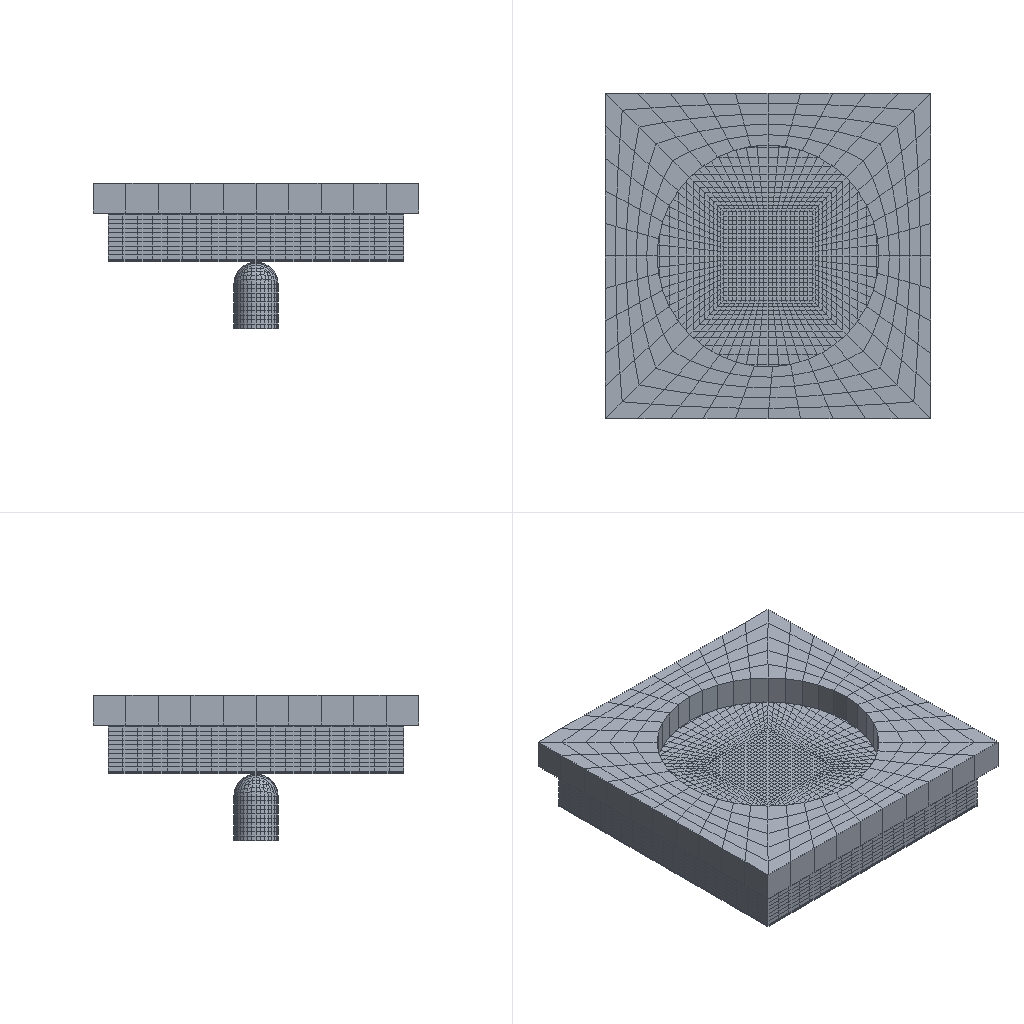Simulation study | abaqus
Set-up summary:
category,name,step,type,value,unit,region
solver,abaqus
solver,version,,,Abaqus/Explicit 2020
units,not stated in the deck,,not stated
analysis,deck,,transient,transient
load_step,Step-1,Step-1,transient
load_step,requested,,,1
mesh,nodes,,,44372
mesh,elements,,,36568
element_type,SC8R,,solid_shell,18240
element_type,C3D8R,,solid,16808
element_type,COH3D8,,cohesive,1520
load,load commands in deck,,count,1
bc,support commands in deck,,count,12
material,CFRP,,in results
material,GANGTI,,in results
material,JIAO,,in results
material,PMI,,in results
check,setup vs results,,match,"per instance, exact: element labels, types and connectivity; labels of the nodes the elements use; coordinates not compared"
Abaqus input file, long lists of numbers shortened:
*Heading
** Job name: Job-1 Model name: Model-1
** Generated by: Abaqus/CAE 2020
*Preprint, echo=NO, model=NO, history=NO, contact=NO
**
** PARTS
**
*Part, name=boligang
*Node
      1,         -25.,          55.,           0.
      2,          10.,          90.,           0.
** (17169 more lines like these left out)
*Element, type=C3D8R
1521,    1,    9,  213,   72, 1562, 1570, 1774, 1633
1522,    9,   10,  214,  213, 1570, 1571, 1775, 1774
** (15198 more lines like these left out)
*Elset, elset=eleset1, generate
 1521,  3040,     1
*Elset, elset=eleset2, generate
 3041,  4560,     1
*Elset, elset=eleset3, generate
 4561,  6080,     1
*Elset, elset=eleset4, generate
 6081,  7600,     1
*Elset, elset=eleset5, generate
 7601,  9120,     1
*Elset, elset=eleset6, generate
  9121,  10640,      1
*Elset, elset=eleset7, generate
 10641,  12160,      1
*Elset, elset=eleset8, generate
 12161,  13680,      1
*Elset, elset=eleset9, generate
 13681,  15200,      1
*Elset, elset=eleset10, generate
 15201,  16720,      1
*Elset, elset=all_plate_elems, generate
  1521,  16720,      1
*Elset, elset=paomo, generate
  1521,  16720,      1
*Elset, elset=_plate_interior_surf_S1, internal, generate
  1521,  16720,      1
*Elset, elset=_plate_interior_surf_S2, internal, generate
  1521,  16720,      1
*Elset, elset=_plate_interior_surf_S3, internal, generate
  1521,  16720,      1
*Elset, elset=_plate_interior_surf_S4, internal, generate
  1521,  16720,      1
*Elset, elset=_plate_interior_surf_S5, internal, generate
  1521,  16720,      1
*Elset, elset=_plate_interior_surf_S6, internal, generate
  1521,  16720,      1
*Surface, type=ELEMENT, name=plate_interior_surf
_plate_interior_surf_S1, S1
_plate_interior_surf_S2, S2
_plate_interior_surf_S4, S4
_plate_interior_surf_S6, S6
_plate_interior_surf_S3, S3
_plate_interior_surf_S5, S5
*Orientation, name=Ori-1
          1.,           0.,           0.,           0.,           1.,           0.
3, 0.
** Section: pmi0
*Solid Section, elset=eleset1, orientation=Ori-1, controls=EC-3, material=pmi
,
*Orientation, name=Ori-2
          1.,           0.,           0.,           0.,           1.,           0.
3, 0.
** Section: pmi0
*Solid Section, elset=eleset2, orientation=Ori-2, controls=EC-3, material=pmi
,
*Orientation, name=Ori-3
          1.,           0.,           0.,           0.,           1.,           0.
3, 0.
** Section: pmi0
*Solid Section, elset=eleset3, orientation=Ori-3, controls=EC-3, material=pmi
,
*Orientation, name=Ori-4
          1.,           0.,           0.,           0.,           1.,           0.
3, 0.
** Section: pmi0
*Solid Section, elset=eleset4, orientation=Ori-4, controls=EC-3, material=pmi
,
*Orientation, name=Ori-5
          1.,           0.,           0.,           0.,           1.,           0.
3, 0.
** Section: pmi0
*Solid Section, elset=eleset5, orientation=Ori-5, controls=EC-3, material=pmi
,
*Orientation, name=Ori-6
          1.,           0.,           0.,           0.,           1.,           0.
3, 0.
** Section: pmi0
*Solid Section, elset=eleset6, orientation=Ori-6, controls=EC-3, material=pmi
,
*Orientation, name=Ori-7
          1.,           0.,           0.,           0.,           1.,           0.
3, 0.
** Section: pmi0
*Solid Section, elset=eleset7, orientation=Ori-7, controls=EC-3, material=pmi
,
*Orientation, name=Ori-8
          1.,           0.,           0.,           0.,           1.,           0.
3, 0.
** Section: pmi0
*Solid Section, elset=eleset8, orientation=Ori-8, controls=EC-3, material=pmi
,
*Orientation, name=Ori-9
          1.,           0.,           0.,           0.,           1.,           0.
3, 0.
** Section: pmi0
*Solid Section, elset=eleset9, orientation=Ori-9, controls=EC-3, material=pmi
,
*Orientation, name=Ori-10
          1.,           0.,           0.,           0.,           1.,           0.
3, 0.
** Region: (pmi0:eleset10), (Controls:EC-3), (Material Orientation:eleset10)
*Elset, elset=_I10, internal
 15201, 15202, 15203, 15204, 15205, 15206, 15207, 15208, 15209, 15210, 15211, 15212, 15213, 15215, 15216, 15217
 15218, 15219, 15220, 15221, 15222, 15223, 15224, 15225, 15226, 15227, 15228, 15229, 15230, 15231, 15232, 15233
** (93 more lines like these left out)
** Section: pmi0
*Solid Section, elset=_I10, orientation=Ori-10, controls=EC-3, material=pmi
,
** Region: (pmi0:eleset10), (Controls:Default), (Material Orientation:eleset10)
*Elset, elset=_I11, internal
 15214,
** Section: pmi0
*Solid Section, elset=_I11, orientation=Ori-10, material=pmi
,
*End Part
**
*Part, name=chongtou
*Node
      1,           0.,           0.,           0.
      2,           0.,           0.,         -7.5
** (1742 more lines like these left out)
*Element, type=C3D8R
  1, 209, 210, 950, 932,  15,  14, 178, 177
  2, 210, 211, 951, 950,  14,  13, 179, 178
** (1406 more lines like these left out)
*Node
   1745,           0.,         -7.5,           0.
*Nset, nset=chongtou-RefPt_, internal
1745,
*Nset, nset=_PickedSet3, internal, generate
    1,  1744,     1
*Elset, elset=_PickedSet3, internal, generate
    1,  1408,     1
** Section: gangti
*Solid Section, elset=_PickedSet3, material=gangti
,
*End Part
**
*Part, name=jiaju
*Node
      1,         -85.,         92.5,          10.
      2,          25.,         92.5,          10.
** (478 more lines like these left out)
*Element, type=C3D8R
 1,  62, 193, 229,  55,   1,  19,  36,   4
 2, 193, 194, 230, 229,  19,  20,  35,  36
** (198 more lines like these left out)
*Nset, nset=_PickedSet2, internal, generate
   1,  480,    1
*Elset, elset=_PickedSet2, internal, generate
   1,  200,    1
** Section: gangti
*Solid Section, elset=_PickedSet2, material=gangti
,
*End Part
**
*Part, name=jiao
*Node
      1,         -25.,          55.,           0.
      2,          10.,          90.,           0.
** (3120 more lines like these left out)
*Element, type=COH3D8
1521,    1,    9,  213,   72, 1562, 1570, 1774, 1633
1522,    9,   10,  214,  213, 1570, 1571, 1775, 1774
** (1518 more lines like these left out)
*Elset, elset=jiao, generate
 1521,  3040,     1
*Elset, elset=_PickedSet10, internal, generate
 1521,  3040,     1
*Elset, elset=jiaoshang, generate
 1521,  3040,     1
*Elset, elset=jiaoxia, generate
 1521,  3040,     1
** Section: jiao
*Cohesive Section, elset=_PickedSet10, controls=EC-2, material=jiao, response=TRACTION SEPARATION
,
*End Part
**
*Part, name=mianban
*Node
      1,         -25.,          55.,           0.
      2,          10.,          90.,           0.
** (10925 more lines like these left out)
*Element, type=SC8R
1521,    1,    9,  213,   72, 1562, 1570, 1774, 1633
1522,    9,   10,  214,  213, 1570, 1571, 1775, 1774
** (9118 more lines like these left out)
*Elset, elset=eleset1, generate
 1521,  3040,     1
*Elset, elset=eleset2, generate
 3041,  4560,     1
*Elset, elset=eleset3, generate
 4561,  6080,     1
*Elset, elset=eleset4, generate
 6081,  7600,     1
*Elset, elset=eleset5, generate
 7601,  9120,     1
*Elset, elset=eleset6, generate
  9121,  10640,      1
*Nset, nset=yueshu
    2,    3,    6,    8,   22,   23,   24,   25,   26,   27,   28,   29,   30,   31,   32,   33
   34,   35,   36,   37,   38,   39,   40,   86,   87,   88,   89,   90,   91,   92,   93,   94
** (33 more lines like these left out)
*Elset, elset=ban, generate
  1521,  10640,      1
*Elset, elset=shang, generate
  1521,  10640,      1
*Elset, elset=_inner_S1, internal
  2641,  2642,  2643,  2644,  2645,  2646,  2647,  2648,  2649,  2650,  2651,  2652,  2653,  2654,  2655,  2656
  2657,  2658,  2659,  2660,  2661,  2662,  2663,  2664,  2665,  2666,  2667,  2668,  2669,  2670,  2671,  2672
** (148 more lines like these left out)
*Elset, elset=_inner_S2, internal
  2641,  2642,  2643,  2644,  2645,  2646,  2647,  2648,  2649,  2650,  2651,  2652,  2653,  2654,  2655,  2656
  2657,  2658,  2659,  2660,  2661,  2662,  2663,  2664,  2665,  2666,  2667,  2668,  2669,  2670,  2671,  2672
** (148 more lines like these left out)
*Elset, elset=_inner_S3, internal
  2661,  2662,  2663,  2664,  2665,  2666,  2667,  2668,  2669,  2670,  2671,  2672,  2673,  2674,  2675,  2676
  2677,  2678,  2679,  2680,  2681,  2682,  2683,  2684,  2685,  2686,  2687,  2688,  2689,  2690,  2691,  2692
** (141 more lines like these left out)
*Elset, elset=_inner_S4, internal
  2641,  2642,  2643,  2644,  2645,  2646,  2647,  2648,  2649,  2650,  2651,  2652,  2653,  2654,  2655,  2656
  2657,  2658,  2659,  2661,  2662,  2663,  2664,  2665,  2666,  2667,  2668,  2669,  2670,  2671,  2672,  2673
** (141 more lines like these left out)
*Elset, elset=_inner_S5, internal
  2641,  2642,  2643,  2644,  2645,  2646,  2647,  2648,  2649,  2650,  2651,  2652,  2653,  2654,  2655,  2656
  2657,  2658,  2659,  2660,  2661,  2662,  2663,  2664,  2665,  2666,  2667,  2668,  2669,  2670,  2671,  2672
** (141 more lines like these left out)
*Elset, elset=_inner_S6, internal
  2642,  2643,  2644,  2645,  2646,  2647,  2648,  2649,  2650,  2651,  2652,  2653,  2654,  2655,  2656,  2657
  2658,  2659,  2660,  2662,  2663,  2664,  2665,  2666,  2667,  2668,  2669,  2670,  2671,  2672,  2673,  2674
** (141 more lines like these left out)
*Surface, type=ELEMENT, name=inner
_inner_S1, S1
_inner_S2, S2
_inner_S4, S4
_inner_S6, S6
_inner_S3, S3
_inner_S5, S5
*Orientation, name=Ori-1
          1.,           0.,           0.,           0.,           1.,           0.
3, 0.
** Region: (CompositeLayup-1-1: Generated From Layup), (Controls:EC-1)
*Elset, elset=CompositeLayup-1-1, generate
 1521,  3040,     1
** Section: CompositeLayup-1-1
*Shell Section, elset=CompositeLayup-1-1, composite, orientation=Ori-1, controls=EC-1, stack direction=3, layup=CompositeLayup-1
0.125, 3, cfrp, 0., Ply-1
*Orientation, name=Ori-4
          1.,           0.,           0.,           0.,           1.,           0.
3, 0.
** Region: (CompositeLayup-1-4: Generated From Layup), (Controls:EC-1)
*Elset, elset=CompositeLayup-1-4, generate
 3041,  4560,     1
** Section: CompositeLayup-1-4
*Shell Section, elset=CompositeLayup-1-4, composite, orientation=Ori-4, controls=EC-1, stack direction=3, layup=CompositeLayup-1
0.125, 3, cfrp, 90., Ply-2
*Orientation, name=Ori-2
          1.,           0.,           0.,           0.,           1.,           0.
3, 0.
** Region: (CompositeLayup-1-2: Generated From Layup), (Controls:EC-1)
*Elset, elset=CompositeLayup-1-2, generate
 4561,  6080,     1
** Section: CompositeLayup-1-2
*Shell Section, elset=CompositeLayup-1-2, composite, orientation=Ori-2, controls=EC-1, stack direction=3, layup=CompositeLayup-1
0.125, 3, cfrp, 0., Ply-3
*Orientation, name=Ori-5
          1.,           0.,           0.,           0.,           1.,           0.
3, 0.
** Region: (CompositeLayup-1-5: Generated From Layup), (Controls:EC-1)
*Elset, elset=CompositeLayup-1-5, generate
 6081,  7600,     1
** Section: CompositeLayup-1-5
*Shell Section, elset=CompositeLayup-1-5, composite, orientation=Ori-5, controls=EC-1, stack direction=3, layup=CompositeLayup-1
0.125, 3, cfrp, 90., Ply-4
*Orientation, name=Ori-3
          1.,           0.,           0.,           0.,           1.,           0.
3, 0.
** Region: (CompositeLayup-1-3: Generated From Layup), (Controls:EC-1)
*Elset, elset=CompositeLayup-1-3, generate
 7601,  9120,     1
** Section: CompositeLayup-1-3
*Shell Section, elset=CompositeLayup-1-3, composite, orientation=Ori-3, controls=EC-1, stack direction=3, layup=CompositeLayup-1
0.125, 3, cfrp, 0., Ply-5
*Orientation, name=Ori-6
          1.,           0.,           0.,           0.,           1.,           0.
3, 0.
** Region: (CompositeLayup-1-6: Generated From Layup), (Controls:EC-1)
*Elset, elset=CompositeLayup-1-6, generate
  9121,  10640,      1
** Section: CompositeLayup-1-6
*Shell Section, elset=CompositeLayup-1-6, composite, orientation=Ori-6, controls=EC-1, stack direction=3, layup=CompositeLayup-1
0.125, 3, cfrp, 90., Ply-6
*End Part
**
*Part, name=mianban2
*Node
      1,         -25.,          55.,           0.
      2,          10.,          90.,           0.
** (10925 more lines like these left out)
*Element, type=SC8R
1521,    1,    9,  213,   72, 1562, 1570, 1774, 1633
1522,    9,   10,  214,  213, 1570, 1571, 1775, 1774
** (9118 more lines like these left out)
*Elset, elset=eleset1, generate
 1521,  3040,     1
*Elset, elset=eleset2, generate
 3041,  4560,     1
*Elset, elset=eleset3, generate
 4561,  6080,     1
*Elset, elset=eleset4, generate
 6081,  7600,     1
*Elset, elset=eleset5, generate
 7601,  9120,     1
*Elset, elset=eleset6, generate
  9121,  10640,      1
*Elset, elset=ban, generate
  1521,  10640,      1
*Nset, nset=yueshu
    2,    3,    6,    8,   22,   23,   24,   25,   26,   27,   28,   29,   30,   31,   32,   33
   34,   35,   36,   37,   38,   39,   40,   86,   87,   88,   89,   90,   91,   92,   93,   94
** (33 more lines like these left out)
*Elset, elset=xia, generate
  1521,  10640,      1
*Elset, elset=_inner_S1, internal
  2641,  2642,  2643,  2644,  2645,  2646,  2647,  2648,  2649,  2650,  2651,  2652,  2653,  2654,  2655,  2656
  2657,  2658,  2659,  2660,  2661,  2662,  2663,  2664,  2665,  2666,  2667,  2668,  2669,  2670,  2671,  2672
** (148 more lines like these left out)
*Elset, elset=_inner_S2, internal
  2641,  2642,  2643,  2644,  2645,  2646,  2647,  2648,  2649,  2650,  2651,  2652,  2653,  2654,  2655,  2656
  2657,  2658,  2659,  2660,  2661,  2662,  2663,  2664,  2665,  2666,  2667,  2668,  2669,  2670,  2671,  2672
** (148 more lines like these left out)
*Elset, elset=_inner_S3, internal
  2661,  2662,  2663,  2664,  2665,  2666,  2667,  2668,  2669,  2670,  2671,  2672,  2673,  2674,  2675,  2676
  2677,  2678,  2679,  2680,  2681,  2682,  2683,  2684,  2685,  2686,  2687,  2688,  2689,  2690,  2691,  2692
** (141 more lines like these left out)
*Elset, elset=_inner_S4, internal
  2641,  2642,  2643,  2644,  2645,  2646,  2647,  2648,  2649,  2650,  2651,  2652,  2653,  2654,  2655,  2656
  2657,  2658,  2659,  2661,  2662,  2663,  2664,  2665,  2666,  2667,  2668,  2669,  2670,  2671,  2672,  2673
** (141 more lines like these left out)
*Elset, elset=_inner_S5, internal
  2641,  2642,  2643,  2644,  2645,  2646,  2647,  2648,  2649,  2650,  2651,  2652,  2653,  2654,  2655,  2656
  2657,  2658,  2659,  2660,  2661,  2662,  2663,  2664,  2665,  2666,  2667,  2668,  2669,  2670,  2671,  2672
** (141 more lines like these left out)
*Elset, elset=_inner_S6, internal
  2642,  2643,  2644,  2645,  2646,  2647,  2648,  2649,  2650,  2651,  2652,  2653,  2654,  2655,  2656,  2657
  2658,  2659,  2660,  2662,  2663,  2664,  2665,  2666,  2667,  2668,  2669,  2670,  2671,  2672,  2673,  2674
** (141 more lines like these left out)
*Surface, type=ELEMENT, name=inner
_inner_S1, S1
_inner_S2, S2
_inner_S4, S4
_inner_S6, S6
_inner_S3, S3
_inner_S5, S5
*Orientation, name=Ori-1
          1.,           0.,           0.,           0.,           1.,           0.
3, 0.
** Region: (CompositeLayup-1-1: Generated From Layup), (Controls:EC-1)
*Elset, elset=CompositeLayup-1-1, generate
 1521,  3040,     1
** Section: CompositeLayup-1-1
*Shell Section, elset=CompositeLayup-1-1, composite, orientation=Ori-1, controls=EC-1, stack direction=3, layup=CompositeLayup-1
0.125, 3, cfrp, 0., Ply-1
*Orientation, name=Ori-4
          1.,           0.,           0.,           0.,           1.,           0.
3, 0.
** Region: (CompositeLayup-1-4: Generated From Layup), (Controls:EC-1)
*Elset, elset=CompositeLayup-1-4, generate
 3041,  4560,     1
** Section: CompositeLayup-1-4
*Shell Section, elset=CompositeLayup-1-4, composite, orientation=Ori-4, controls=EC-1, stack direction=3, layup=CompositeLayup-1
0.125, 3, cfrp, 90., Ply-2
*Orientation, name=Ori-2
          1.,           0.,           0.,           0.,           1.,           0.
3, 0.
** Region: (CompositeLayup-1-2: Generated From Layup), (Controls:EC-1)
*Elset, elset=CompositeLayup-1-2, generate
 4561,  6080,     1
** Section: CompositeLayup-1-2
*Shell Section, elset=CompositeLayup-1-2, composite, orientation=Ori-2, controls=EC-1, stack direction=3, layup=CompositeLayup-1
0.125, 3, cfrp, 0., Ply-3
*Orientation, name=Ori-5
          1.,           0.,           0.,           0.,           1.,           0.
3, 0.
** Region: (CompositeLayup-1-5: Generated From Layup), (Controls:EC-1)
*Elset, elset=CompositeLayup-1-5, generate
 6081,  7600,     1
** Section: CompositeLayup-1-5
*Shell Section, elset=CompositeLayup-1-5, composite, orientation=Ori-5, controls=EC-1, stack direction=3, layup=CompositeLayup-1
0.125, 3, cfrp, 90., Ply-4
*Orientation, name=Ori-3
          1.,           0.,           0.,           0.,           1.,           0.
3, 0.
** Region: (CompositeLayup-1-3: Generated From Layup), (Controls:EC-1)
*Elset, elset=CompositeLayup-1-3, generate
 7601,  9120,     1
** Section: CompositeLayup-1-3
*Shell Section, elset=CompositeLayup-1-3, composite, orientation=Ori-3, controls=EC-1, stack direction=3, layup=CompositeLayup-1
0.125, 3, cfrp, 0., Ply-5
*Orientation, name=Ori-6
          1.,           0.,           0.,           0.,           1.,           0.
3, 0.
** Region: (CompositeLayup-1-6: Generated From Layup), (Controls:EC-1)
*Elset, elset=CompositeLayup-1-6, generate
  9121,  10640,      1
** Section: CompositeLayup-1-6
*Shell Section, elset=CompositeLayup-1-6, composite, orientation=Ori-6, controls=EC-1, stack direction=3, layup=CompositeLayup-1
0.125, 3, cfrp, 90., Ply-6
*End Part
**
**
** ASSEMBLY
**
*Assembly, name=Assembly
**
*Instance, name=chongtou-1, part=chongtou
        -35.,         42.5,       -24.05
        -35.,         42.5,       -24.05, -36.,         42.5,       -24.05, 90.
*End Instance
**
*Instance, name=jiaju-1, part=jiaju
         -5.,           5.,           0.
*End Instance
**
*Instance, name=mianban-1, part=mianban
          5.,          2.5,        -16.5
*End Instance
**
*Instance, name=mianban2-1, part=mianban2
          5.,          2.5,        -0.75
*End Instance
**
*Instance, name=jiao-1, part=jiao
          5.,          2.5,       -15.75
*End Instance
**
*Instance, name=boligang-1, part=boligang
          5.,          2.5,       -15.65
*End Instance
**
*Node
      1,         -35.,         42.5,          10.
*Elset, elset=ban, instance=mianban2-1, generate
  1521,  10640,      1
*Nset, nset=tou, instance=chongtou-1
 1745,
*Nset, nset=_PickedSet13, internal, instance=chongtou-1
 1745,
*Nset, nset=_PickedSet17, internal
 1,
*Nset, nset=_PickedSet18, internal, instance=jiaju-1, generate
   1,  480,    1
*Elset, elset=_PickedSet18, internal, instance=jiaju-1, generate
   1,  200,    1
*Nset, nset=_PickedSet19, internal
 1,
*Nset, nset=_PickedSet20, internal, instance=chongtou-1
 1745,
*Nset, nset=_PickedSet44, internal, instance=chongtou-1, generate
    1,  1744,     1
*Elset, elset=_PickedSet44, internal, instance=chongtou-1, generate
    1,  1408,     1
*Nset, nset=_PickedSet83, internal, instance=mianban2-1
    2,    3,    6,    8,   22,   23,   24,   25,   26,   27,   28,   29,   30,   31,   32,   33
   34,   35,   36,   37,   38,   39,   40,   86,   87,   88,   89,   90,   91,   92,   93,   94
** (33 more lines like these left out)
*Nset, nset=_PickedSet83, internal, instance=boligang-1
     2,     3,     6,     8,    22,    23,    24,    25,    26,    27,    28,    29,    30,    31,    32,    33
    34,    35,    36,    37,    38,    39,    40,    86,    87,    88,    89,    90,    91,    92,    93,    94
** (53 more lines like these left out)
*Elset, elset=_inner_S1, internal, instance=mianban2-1
  1521,  1522,  1523,  1524,  1535,  1536,  1537,  1538,  1549,  1550,  1551,  1552,  1563,  1564,  1565,  1566
  1577,  1578,  1579,  1580,  1591,  1592,  1593,  1594,  1605,  1606,  1607,  1608,  1619,  1620,  1621,  1622
** (268 more lines like these left out)
*Elset, elset=_inner_S1, internal, instance=boligang-1
  1521,  1522,  1523,  1535,  1536,  1537,  1549,  1550,  1551,  1563,  1564,  1565,  1577,  1578,  1579,  1591
  1592,  1593,  1605,  1606,  1607,  1619,  1620,  1621,  1633,  1634,  1635,  1647,  1648,  1649,  1661,  1662
** (426 more lines like these left out)
*Elset, elset=_inner_S2, internal, instance=mianban2-1
  1521,  1522,  1523,  1524,  1535,  1536,  1537,  1538,  1549,  1550,  1551,  1552,  1563,  1564,  1565,  1566
  1577,  1578,  1579,  1580,  1591,  1592,  1593,  1594,  1605,  1606,  1607,  1608,  1619,  1620,  1621,  1622
** (268 more lines like these left out)
*Elset, elset=_inner_S2, internal, instance=boligang-1
  1521,  1522,  1523,  1535,  1536,  1537,  1549,  1550,  1551,  1563,  1564,  1565,  1577,  1578,  1579,  1591
  1592,  1593,  1605,  1606,  1607,  1619,  1620,  1621,  1633,  1634,  1635,  1647,  1648,  1649,  1661,  1662
** (431 more lines like these left out)
*Elset, elset=_inner_S3, internal, instance=mianban2-1
  1521,  1522,  1523,  1535,  1536,  1537,  1538,  1549,  1550,  1551,  1552,  1563,  1564,  1565,  1566,  1577
  1578,  1579,  1580,  1591,  1592,  1593,  1594,  1605,  1606,  1607,  1608,  1619,  1620,  1621,  1622,  1633
** (267 more lines like these left out)
*Elset, elset=_inner_S3, internal, instance=boligang-1
  1521,  1522,  1523,  1535,  1536,  1537,  1549,  1550,  1551,  1563,  1564,  1565,  1577,  1578,  1579,  1591
  1592,  1593,  1605,  1606,  1607,  1619,  1620,  1621,  1633,  1634,  1635,  1647,  1648,  1649,  1661,  1662
** (430 more lines like these left out)
*Elset, elset=_inner_S4, internal, instance=mianban2-1
  1521,  1522,  1523,  1535,  1536,  1537,  1549,  1550,  1551,  1563,  1564,  1565,  1577,  1578,  1579,  1591
  1592,  1593,  1605,  1606,  1607,  1619,  1620,  1621,  1633,  1634,  1635,  1647,  1648,  1649,  1661,  1662
** (253 more lines like these left out)
*Elset, elset=_inner_S4, internal, instance=boligang-1
  1521,  1522,  1535,  1536,  1549,  1550,  1563,  1564,  1577,  1578,  1591,  1592,  1605,  1606,  1619,  1620
  1633,  1634,  1647,  1648,  1661,  1662,  1675,  1676,  1689,  1690,  1703,  1704,  1717,  1718,  1731,  1732
** (406 more lines like these left out)
*Elset, elset=_inner_S5, internal, instance=mianban2-1
  1521,  1522,  1523,  1524,  1535,  1536,  1537,  1538,  1549,  1550,  1551,  1552,  1563,  1564,  1565,  1566
  1577,  1578,  1579,  1580,  1591,  1592,  1593,  1594,  1605,  1606,  1607,  1608,  1619,  1620,  1621,  1622
** (268 more lines like these left out)
*Elset, elset=_inner_S5, internal, instance=boligang-1
  1521,  1522,  1523,  1535,  1536,  1537,  1549,  1550,  1551,  1563,  1564,  1565,  1577,  1578,  1579,  1591
  1592,  1593,  1605,  1606,  1607,  1619,  1620,  1621,  1633,  1634,  1635,  1647,  1648,  1649,  1661,  1662
** (430 more lines like these left out)
*Elset, elset=_inner_S6, internal, instance=mianban2-1
  1521,  1522,  1523,  1524,  1535,  1536,  1537,  1538,  1549,  1550,  1551,  1552,  1563,  1564,  1565,  1566
  1577,  1578,  1579,  1580,  1591,  1592,  1593,  1594,  1605,  1606,  1607,  1608,  1619,  1620,  1621,  1622
** (253 more lines like these left out)
*Elset, elset=_inner_S6, internal, instance=boligang-1
  1521,  1522,  1523,  1535,  1536,  1537,  1549,  1550,  1551,  1563,  1564,  1565,  1577,  1578,  1579,  1591
  1592,  1593,  1605,  1606,  1607,  1619,  1620,  1621,  1633,  1634,  1635,  1647,  1648,  1649,  1661,  1662
** (406 more lines like these left out)
*Surface, type=ELEMENT, name=inner
_inner_S1, S1
_inner_S2, S2
_inner_S4, S4
_inner_S6, S6
_inner_S3, S3
_inner_S5, S5
*Elset, elset=_mian_S3, internal, instance=chongtou-1
   65,   66,   67,   68,   69,   70,   71,   72,   73,   74,   75,   76,   77,   78,   79,   80
   97,   98,   99,  100,  101,  102,  103,  104,  105,  106,  107,  108,  109,  110,  111,  112
** (2 more lines like these left out)
*Elset, elset=_mian_S4, internal, instance=chongtou-1
   81,   82,   83,   84,   85,   86,   87,   88,   89,   90,   91,   92,   93,   94,   95,   96
  465,  466,  467,  468,  469,  470,  471,  472,  473,  474,  475,  476,  477,  478,  479,  480
** (3 more lines like these left out)
*Elset, elset=_mian_S2, internal, instance=chongtou-1, generate
 353,  400,    1
*Surface, type=ELEMENT, name=mian
_mian_S3, S3
_mian_S4, S4
_mian_S2, S2
*Elset, elset=_s_Surf-9_S2, internal, instance=jiao-1, generate
 1521,  3040,     1
*Surface, type=ELEMENT, name=s_Surf-9
_s_Surf-9_S2, S2
*Elset, elset=__PickedSurf71_S1, internal, instance=boligang-1, generate
 1521,  3040,     1
*Surface, type=ELEMENT, name=_PickedSurf71, internal
__PickedSurf71_S1, S1
*Elset, elset=__PickedSurf75_S2, internal, instance=boligang-1, generate
 15201,  16720,      1
*Surface, type=ELEMENT, name=_PickedSurf75, internal
__PickedSurf75_S2, S2
*Elset, elset=__PickedSurf76_S1, internal, instance=mianban2-1, generate
 1521,  3040,     1
*Surface, type=ELEMENT, name=_PickedSurf76, internal
__PickedSurf76_S1, S1
** Constraint: Constraint-1
*Rigid Body, ref node=_PickedSet13, elset=_PickedSet44, position=CENTER OF MASS
** Constraint: Constraint-2
*Rigid Body, ref node=_PickedSet17, elset=_PickedSet18, position=CENTER OF MASS
** Constraint: Constraint-3
*Tie, name=Constraint-3, adjust=yes
s_Surf-9, _PickedSurf71
** Constraint: Constraint-5
*Tie, name=Constraint-5, adjust=yes
_PickedSurf76, _PickedSurf75
*End Assembly
**
** ELEMENT CONTROLS
**
*Section Controls, name=EC-1, ELEMENT DELETION=YES, MAX DEGRADATION=0.9, hourglass=ENHANCED
1., 1., 1.
*Section Controls, name=EC-2, ELEMENT DELETION=YES, MAX DEGRADATION=0.9
1., 1., 1.
*Section Controls, name=EC-3, hourglass=ENHANCED
1., 1., 1.
**
** MATERIALS
**
*Material, name=cfrp
*Damage Initiation, criterion=HASHIN
2537.,1580.,  82., 236.,  90.,  40.
*Damage Evolution, type=ENERGY
 91.6, 79.9, 0.22,  1.1
*Density
 1.6e-09,
*Elastic, type=LAMINA
153000.,10300.,   0.3, 6000., 6000., 3700.
*Material, name=gangti
*Density
 2.82929e-07,
*Elastic
210000., 0.3
*Material, name=jiao
*Damage Initiation, criterion=QUADS
30.,50.,50.
*Damage Evolution, type=ENERGY, mixed mode behavior=BK, power=1.45
 0.28, 0.79, 0.79
*Density
 1.6e-09,
*Elastic, type=TRACTION
100000.,100000.,100000.
*Material, name=pmi
*Density
 5.1e-09,
*Elastic
100000., 0.35
**
** INTERACTION PROPERTIES
**
*Surface Interaction, name=IntProp-1
*Friction
 0.15,
*Surface Behavior, pressure-overclosure=HARD
**
** BOUNDARY CONDITIONS
**
** Name: BC-1 Type: 对称/反对称/完全固定
*Boundary
_PickedSet19, ENCASTRE
** Name: BC-2 Type: 位移/转角
*Boundary
_PickedSet20, 1, 1
_PickedSet20, 2, 2
_PickedSet20, 4, 4
_PickedSet20, 5, 5
_PickedSet20, 6, 6
** Name: BC-3 Type: 位移/转角
*Boundary
_PickedSet83, 1, 1
_PickedSet83, 2, 2
_PickedSet83, 3, 3
_PickedSet83, 4, 4
_PickedSet83, 5, 5
_PickedSet83, 6, 6
**
** PREDEFINED FIELDS
**
** Name: Predefined Field-1   Type: Velocity
*Initial Conditions, type=VELOCITY
tou, 1, 0.
tou, 2, 0.
tou, 3, 5477.23
** ----------------------------------------------------------------
**
** STEP: Step-1
**
*Step, name=Step-1, nlgeom=YES
*Dynamic, Explicit, element by element
, 0.005
*Bulk Viscosity
0.06, 1.2
** Mass Scaling: Semi-Automatic
**               Whole Model
*Fixed Mass Scaling, factor=5000.
**
** INTERACTIONS
**
** Interaction: Int-1
*Contact, op=NEW
*Contact Inclusions
 ,
 , inner
inner ,
*Contact Property Assignment
 ,  , IntProp-1
**
** OUTPUT REQUESTS
**
*Restart, write, number interval=1, time marks=NO
**
** FIELD OUTPUT: F-Output-1
**
*Output, field, number interval=100
*Node Output
A, RF, RM, RT, U, V
*Element Output, directions=YES
DMICRT, E, EVF, FV, LE, MISES, PE, PEEQ, PEEQVAVG, PEVAVG, S, SDEG, SDV, STATUS, SVAVG
*Contact Output
CSTRESS,
**
** FIELD OUTPUT: F-Output-2
**
*Element Output, elset=mianban-1.CompositeLayup-1-1, directions=YES
2
DAMAGEC, DAMAGEFC, DAMAGEFT, DAMAGEMC, DAMAGEMT, DAMAGESHR, DAMAGET, DMICRT, S, SDEG
**
** FIELD OUTPUT: F-Output-3
**
*Element Output, elset=mianban2-1.CompositeLayup-1-1, directions=YES
2
DAMAGEC, DAMAGEFC, DAMAGEFT, DAMAGEMC, DAMAGEMT, DAMAGESHR, DAMAGET, DMICRT, S, SDEG, SDV, STATUS
**
** FIELD OUTPUT: F-Output-2
**
*Element Output, elset=mianban-1.CompositeLayup-1-2, directions=YES
2
DAMAGEC, DAMAGEFC, DAMAGEFT, DAMAGEMC, DAMAGEMT, DAMAGESHR, DAMAGET, DMICRT, S, SDEG
**
** FIELD OUTPUT: F-Output-3
**
*Element Output, elset=mianban2-1.CompositeLayup-1-2, directions=YES
2
DAMAGEC, DAMAGEFC, DAMAGEFT, DAMAGEMC, DAMAGEMT, DAMAGESHR, DAMAGET, DMICRT, S, SDEG, SDV, STATUS
**
** FIELD OUTPUT: F-Output-2
**
*Element Output, elset=mianban-1.CompositeLayup-1-3, directions=YES
2
DAMAGEC, DAMAGEFC, DAMAGEFT, DAMAGEMC, DAMAGEMT, DAMAGESHR, DAMAGET, DMICRT, S, SDEG
**
** FIELD OUTPUT: F-Output-3
**
*Element Output, elset=mianban2-1.CompositeLayup-1-3, directions=YES
2
DAMAGEC, DAMAGEFC, DAMAGEFT, DAMAGEMC, DAMAGEMT, DAMAGESHR, DAMAGET, DMICRT, S, SDEG, SDV, STATUS
**
** FIELD OUTPUT: F-Output-2
**
*Element Output, elset=mianban-1.CompositeLayup-1-4, directions=YES
2
DAMAGEC, DAMAGEFC, DAMAGEFT, DAMAGEMC, DAMAGEMT, DAMAGESHR, DAMAGET, DMICRT, S, SDEG
**
** FIELD OUTPUT: F-Output-3
**
*Element Output, elset=mianban2-1.CompositeLayup-1-4, directions=YES
2
DAMAGEC, DAMAGEFC, DAMAGEFT, DAMAGEMC, DAMAGEMT, DAMAGESHR, DAMAGET, DMICRT, S, SDEG, SDV, STATUS
**
** FIELD OUTPUT: F-Output-2
**
*Element Output, elset=mianban-1.CompositeLayup-1-5, directions=YES
2
DAMAGEC, DAMAGEFC, DAMAGEFT, DAMAGEMC, DAMAGEMT, DAMAGESHR, DAMAGET, DMICRT, S, SDEG
**
** FIELD OUTPUT: F-Output-3
**
*Element Output, elset=mianban2-1.CompositeLayup-1-5, directions=YES
2
DAMAGEC, DAMAGEFC, DAMAGEFT, DAMAGEMC, DAMAGEMT, DAMAGESHR, DAMAGET, DMICRT, S, SDEG, SDV, STATUS
**
** FIELD OUTPUT: F-Output-2
**
*Element Output, elset=mianban-1.CompositeLayup-1-6, directions=YES
2
DAMAGEC, DAMAGEFC, DAMAGEFT, DAMAGEMC, DAMAGEMT, DAMAGESHR, DAMAGET, DMICRT, S, SDEG
**
** FIELD OUTPUT: F-Output-3
**
*Element Output, elset=mianban2-1.CompositeLayup-1-6, directions=YES
2
DAMAGEC, DAMAGEFC, DAMAGEFT, DAMAGEMC, DAMAGEMT, DAMAGESHR, DAMAGET, DMICRT, S, SDEG, SDV, STATUS
**
** HISTORY OUTPUT: ban
**
*Output, history, time interval=5e-05
*Energy Output, elset=ban
ALLAE, ALLCD, ALLCW, ALLDC, ALLDMD, ALLFD, ALLIE, ALLKE, ALLMW, ALLPD, ALLPW, ALLSE, ALLVD, ALLWK, ETOTAL
**
** HISTORY OUTPUT: weiyi
**
*Node Output, nset=tou
A3, U3, V3
**
** HISTORY OUTPUT: nengliang
**
*Output, history
*Energy Output
ALLAE, ALLCD, ALLCW, ALLDC, ALLDMD, ALLFD, ALLIE, ALLKE, ALLMW, ALLPD, ALLPW, ALLSE, ALLVD, ALLWK, ETOTAL
**
** HISTORY OUTPUT: li
**
*Contact Output, surface=mian
CFN1, CFN2, CFN3, CFNM, CFS1, CFS2, CFS3, CFSM
**
** HISTORY OUTPUT: shangban
**
*Energy Output, elset=mianban-1.shang
ALLAE, ALLIE, ALLKE, ETOTAL
**
** HISTORY OUTPUT: xiaban
**
*Energy Output, elset=mianban2-1.xia
ALLAE, ALLIE, ALLKE, ETOTAL
*End Step
Results summary:
result,step,Step-1,completed,increments=18869 time=0.005/0.005
result,analysis,,,transient
result,last_loadstep,,,1
result,primary field,,,U
result,reaction total,,FX,127938.377,model units
result,reaction total,,FY,101534.601,model units
result,reaction total,,FZ,-5615244.954,model units